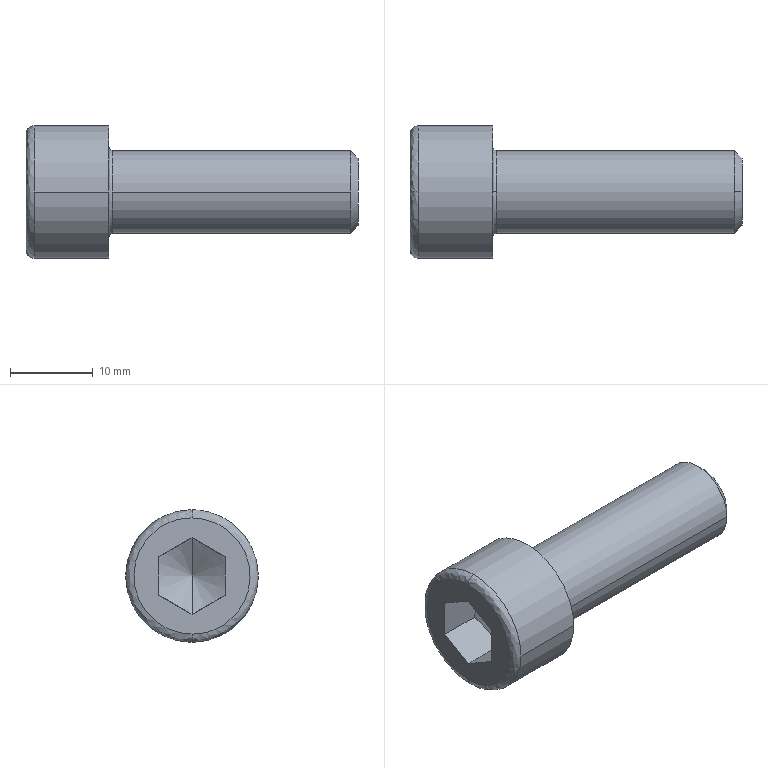Part | STEP file | Broached Socket Head Cap Screw - Metric M10x1.5 x 30 | 1 solid | 21 faces | box 40 x 16 x 16 mm | volume 4010 mm3 | plane 9 | spline 4 | cylinder 4 | cone 4 | commonest cylinder face diameters 10 x2 16 x2